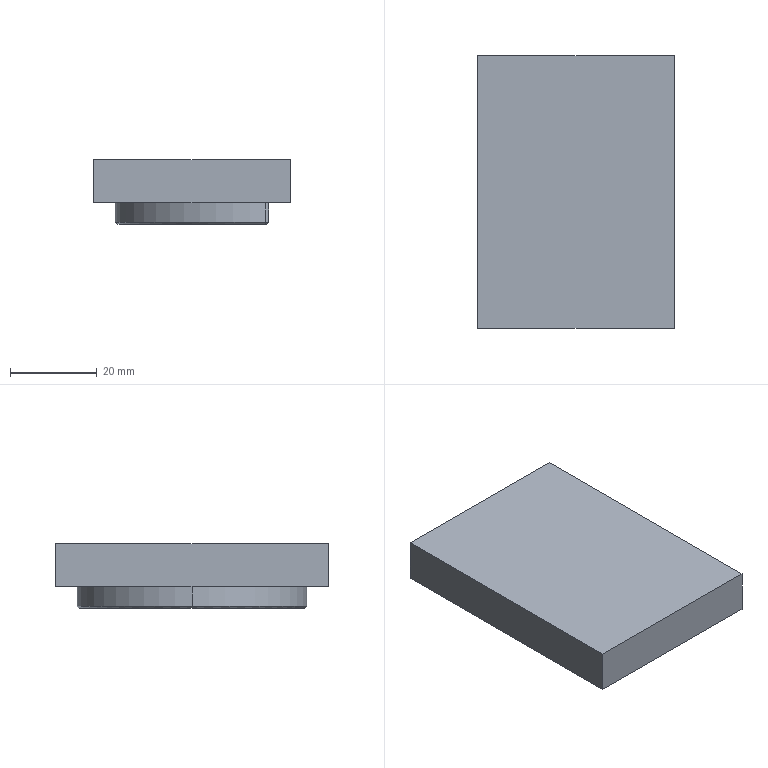Part | 2 solids | 72 faces | box 45.394 x 63 x 15 mm | volume 30952 mm3 | cylinder 32 | plane 22 | cone 18 | commonest cylinder face diameters 3.4 x8 6 x8 10 x4 37 x3 53 x3 2 x2